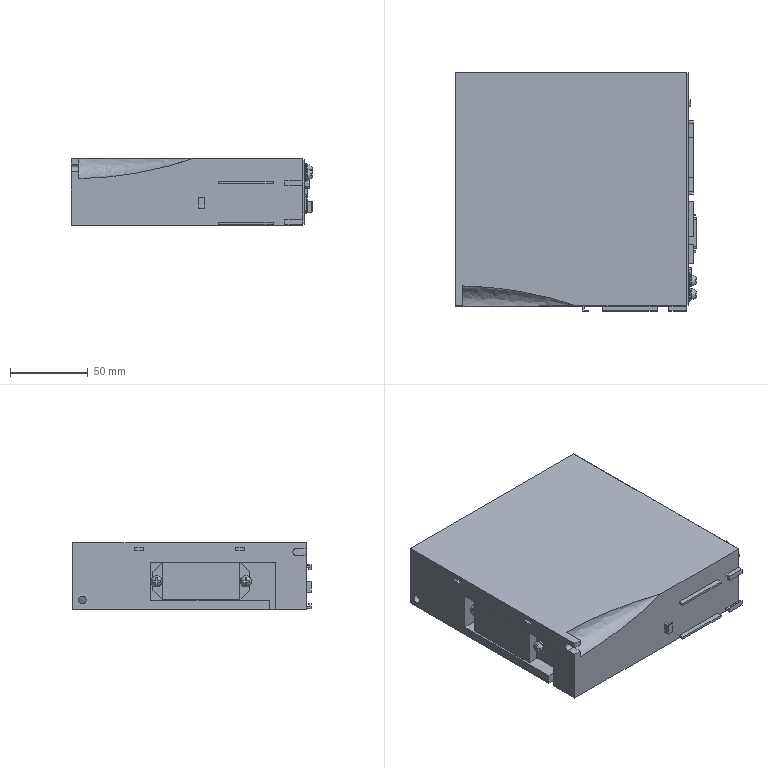Part | STEP file | ME30_E-RAM6-S-640-ME30-C5 | 1 solid | 901 faces | box 155.627 x 153.2 x 43 mm | volume 932829 mm3 | plane 734 | cylinder 121 | cone 20 | torus 20 | sphere 4 | spline 2 | commonest cylinder face diameters 3.1 x24 1 x20 2 x9 0.4 x4 1.2 x4 1.56 x4